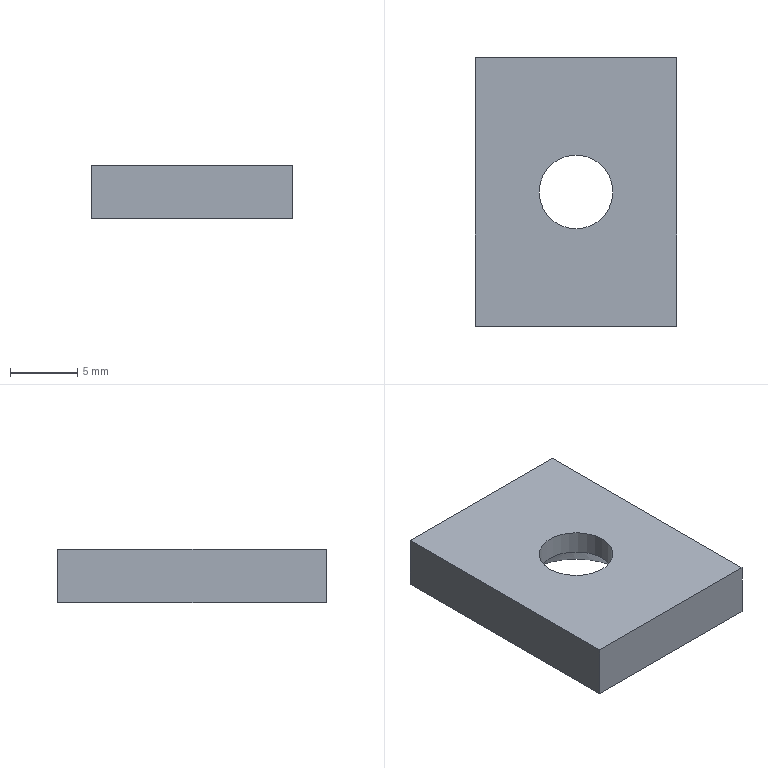Part | NX | features DATUM_CSYS 2, CSUNK_HOLE 1, EXTRUDE 1, HOLE PACKAGE 1, SKETCH 1 | 1 solid | 8 faces | box 15 x 20 x 4 mm | volume 1049 mm3 | plane 6 | cylinder 1 | cone 1 | commonest cylinder face diameters 5.5 x1
STEP:
#1=CARTESIAN_POINT('',(-7.5,10.,0.));
#2=VERTEX_POINT('',#1);
#3=CARTESIAN_POINT('',(-7.5,-10.,0.));
#4=VERTEX_POINT('',#3);
#5=CARTESIAN_POINT('',(-7.5,10.,0.));
#6=DIRECTION('',(0.,-1.,0.));
#7=VECTOR('',#6,1000.);
#8=LINE('',#5,#7);
#9=EDGE_CURVE('',#2,#4,#8,.T.);
#10=ORIENTED_EDGE('',*,*,#9,.T.);
#11=CARTESIAN_POINT('',(-7.5,-10.,4.));
#12=VERTEX_POINT('',#11);
#13=CARTESIAN_POINT('',(-7.5,-10.,4.));
#14=DIRECTION('',(0.,0.,-1.));
#15=VECTOR('',#14,1000.);
#16=LINE('',#13,#15);
#17=EDGE_CURVE('',#12,#4,#16,.T.);
#18=ORIENTED_EDGE('',*,*,#17,.F.);
#19=CARTESIAN_POINT('',(-7.5,10.,4.));
#20=VERTEX_POINT('',#19);
#21=CARTESIAN_POINT('',(-7.5,10.,4.));
#22=DIRECTION('',(0.,-1.,0.));
#23=VECTOR('',#22,1000.);
#24=LINE('',#21,#23);
#25=EDGE_CURVE('',#20,#12,#24,.T.);
#26=ORIENTED_EDGE('',*,*,#25,.F.);
#27=CARTESIAN_POINT('',(-7.5,10.,4.));
#28=DIRECTION('',(0.,0.,-1.));
#29=VECTOR('',#28,1000.);
#30=LINE('',#27,#29);
#31=EDGE_CURVE('',#20,#2,#30,.T.);
#32=ORIENTED_EDGE('',*,*,#31,.T.);
#33=EDGE_LOOP('',(#10,#18,#26,#32));
#34=FACE_BOUND('',#33,.T.);
#35=CARTESIAN_POINT('',(-7.5,10.,4.));
#36=DIRECTION('',(1.,0.,0.));
#37=DIRECTION('',(0.,1.,0.));
#38=AXIS2_PLACEMENT_3D('',#35,#36,#37);
#39=PLANE('',#38);
#40=ADVANCED_FACE('',(#34),#39,.F.);
#41=CARTESIAN_POINT('',(7.5,-10.,0.));
#42=VERTEX_POINT('',#41);
#43=CARTESIAN_POINT('',(-7.5,-10.,0.));
#44=DIRECTION('',(1.,0.,0.));
#45=VECTOR('',#44,1000.);
#46=LINE('',#43,#45);
#47=EDGE_CURVE('',#4,#42,#46,.T.);
#48=ORIENTED_EDGE('',*,*,#47,.T.);
#49=CARTESIAN_POINT('',(7.5,-10.,4.));
#50=VERTEX_POINT('',#49);
#51=CARTESIAN_POINT('',(7.5,-10.,4.));
#52=DIRECTION('',(0.,0.,-1.));
#53=VECTOR('',#52,1000.);
#54=LINE('',#51,#53);
#55=EDGE_CURVE('',#50,#42,#54,.T.);
#56=ORIENTED_EDGE('',*,*,#55,.F.);
#57=CARTESIAN_POINT('',(-7.5,-10.,4.));
#58=DIRECTION('',(1.,0.,0.));
#59=VECTOR('',#58,1000.);
#60=LINE('',#57,#59);
#61=EDGE_CURVE('',#12,#50,#60,.T.);
#62=ORIENTED_EDGE('',*,*,#61,.F.);
#63=ORIENTED_EDGE('',*,*,#17,.T.);
#64=EDGE_LOOP('',(#48,#56,#62,#63));
#65=FACE_BOUND('',#64,.T.);
#66=CARTESIAN_POINT('',(-7.5,-10.,4.));
#67=DIRECTION('',(0.,1.,0.));
#68=DIRECTION('',(-1.,0.,0.));
#69=AXIS2_PLACEMENT_3D('',#66,#67,#68);
#70=PLANE('',#69);
#71=ADVANCED_FACE('',(#65),#70,.F.);
#72=CARTESIAN_POINT('',(7.5,10.,0.));
#73=VERTEX_POINT('',#72);
#74=CARTESIAN_POINT('',(7.5,-10.,0.));
#75=DIRECTION('',(0.,1.,0.));
#76=VECTOR('',#75,1000.);
#77=LINE('',#74,#76);
#78=EDGE_CURVE('',#42,#73,#77,.T.);
#79=ORIENTED_EDGE('',*,*,#78,.T.);
#80=CARTESIAN_POINT('',(7.5,10.,4.));
#81=VERTEX_POINT('',#80);
#82=CARTESIAN_POINT('',(7.5,10.,4.));
#83=DIRECTION('',(0.,0.,-1.));
#84=VECTOR('',#83,1000.);
#85=LINE('',#82,#84);
#86=EDGE_CURVE('',#81,#73,#85,.T.);
#87=ORIENTED_EDGE('',*,*,#86,.F.);
#88=CARTESIAN_POINT('',(7.5,-10.,4.));
#89=DIRECTION('',(0.,1.,0.));
#90=VECTOR('',#89,1000.);
#91=LINE('',#88,#90);
#92=EDGE_CURVE('',#50,#81,#91,.T.);
#93=ORIENTED_EDGE('',*,*,#92,.F.);
#94=ORIENTED_EDGE('',*,*,#55,.T.);
#95=EDGE_LOOP('',(#79,#87,#93,#94));
#96=FACE_BOUND('',#95,.T.);
#97=CARTESIAN_POINT('',(7.5,-10.,4.));
#98=DIRECTION('',(-1.,0.,0.));
#99=DIRECTION('',(0.,-1.,0.));
#100=AXIS2_PLACEMENT_3D('',#97,#98,#99);
#101=PLANE('',#100);
#102=ADVANCED_FACE('',(#96),#101,.F.);
#103=CARTESIAN_POINT('',(7.5,10.,0.));
#104=DIRECTION('',(-1.,0.,0.));
#105=VECTOR('',#104,1000.);
#106=LINE('',#103,#105);
#107=EDGE_CURVE('',#73,#2,#106,.T.);
#108=ORIENTED_EDGE('',*,*,#107,.T.);
#109=ORIENTED_EDGE('',*,*,#31,.F.);
#110=CARTESIAN_POINT('',(7.5,10.,4.));
#111=DIRECTION('',(-1.,0.,0.));
#112=VECTOR('',#111,1000.);
#113=LINE('',#110,#112);
#114=EDGE_CURVE('',#81,#20,#113,.T.);
#115=ORIENTED_EDGE('',*,*,#114,.F.);
#116=ORIENTED_EDGE('',*,*,#86,.T.);
#117=EDGE_LOOP('',(#108,#109,#115,#116));
#118=FACE_BOUND('',#117,.T.);
#119=CARTESIAN_POINT('',(7.5,10.,4.));
#120=DIRECTION('',(0.,-1.,0.));
#121=DIRECTION('',(1.,0.,0.));
#122=AXIS2_PLACEMENT_3D('',#119,#120,#121);
#123=PLANE('',#122);
#124=ADVANCED_FACE('',(#118),#123,.F.);
#125=CARTESIAN_POINT('',(2.75,0.,4.));
#126=VERTEX_POINT('',#125);
#127=CARTESIAN_POINT('',(0.,0.,4.));
#128=DIRECTION('',(0.,0.,1.));
#129=DIRECTION('',(1.,0.,0.));
#130=AXIS2_PLACEMENT_3D('',#127,#128,#129);
#131=CIRCLE('',#130,2.75);
#132=EDGE_CURVE('',#126,#126,#131,.T.);
#133=ORIENTED_EDGE('',*,*,#132,.F.);
#134=EDGE_LOOP('',(#133));
#135=FACE_BOUND('',#134,.T.);
#136=ORIENTED_EDGE('',*,*,#25,.T.);
#137=ORIENTED_EDGE('',*,*,#61,.T.);
#138=ORIENTED_EDGE('',*,*,#92,.T.);
#139=ORIENTED_EDGE('',*,*,#114,.T.);
#140=EDGE_LOOP('',(#136,#137,#138,#139));
#141=FACE_BOUND('',#140,.T.);
#142=CARTESIAN_POINT('',(0.,0.,4.));
#143=DIRECTION('',(0.,0.,1.));
#144=DIRECTION('',(1.,0.,0.));
#145=AXIS2_PLACEMENT_3D('',#142,#143,#144);
#146=PLANE('',#145);
#147=ADVANCED_FACE('',(#135,#141),#146,.T.);
#148=CARTESIAN_POINT('',(5.,0.,0.));
#149=VERTEX_POINT('',#148);
#150=CARTESIAN_POINT('',(0.,0.,0.));
#151=DIRECTION('',(0.,0.,1.));
#152=DIRECTION('',(1.,0.,0.));
#153=AXIS2_PLACEMENT_3D('',#150,#151,#152);
#154=CIRCLE('',#153,5.);
#155=EDGE_CURVE('',#149,#149,#154,.T.);
#156=ORIENTED_EDGE('',*,*,#155,.T.);
#157=EDGE_LOOP('',(#156));
#158=FACE_BOUND('',#157,.T.);
#159=ORIENTED_EDGE('',*,*,#9,.F.);
#160=ORIENTED_EDGE('',*,*,#107,.F.);
#161=ORIENTED_EDGE('',*,*,#78,.F.);
#162=ORIENTED_EDGE('',*,*,#47,.F.);
#163=EDGE_LOOP('',(#159,#160,#161,#162));
#164=FACE_BOUND('',#163,.T.);
#165=CARTESIAN_POINT('',(0.,0.,0.));
#166=DIRECTION('',(0.,0.,1.));
#167=DIRECTION('',(1.,0.,0.));
#168=AXIS2_PLACEMENT_3D('',#165,#166,#167);
#169=PLANE('',#168);
#170=ADVANCED_FACE('',(#158,#164),#169,.F.);
#171=ORIENTED_EDGE('',*,*,#132,.T.);
#172=EDGE_LOOP('',(#171));
#173=FACE_BOUND('',#172,.T.);
#174=CARTESIAN_POINT('',(2.75,0.,2.25));
#175=VERTEX_POINT('',#174);
#176=CARTESIAN_POINT('',(0.,0.,2.25));
#177=DIRECTION('',(0.,0.,1.));
#178=DIRECTION('',(1.,0.,0.));
#179=AXIS2_PLACEMENT_3D('',#176,#177,#178);
#180=CIRCLE('',#179,2.75);
#181=EDGE_CURVE('',#175,#175,#180,.F.);
#182=ORIENTED_EDGE('',*,*,#181,.T.);
#183=EDGE_LOOP('',(#182));
#184=FACE_BOUND('',#183,.T.);
#185=CARTESIAN_POINT('',(0.,0.,15.925));
#186=DIRECTION('',(0.,0.,1.));
#187=DIRECTION('',(1.,0.,0.));
#188=AXIS2_PLACEMENT_3D('',#185,#186,#187);
#189=CYLINDRICAL_SURFACE('',#188,2.75);
#190=ADVANCED_FACE('',(#173,#184),#189,.F.);
#191=ORIENTED_EDGE('',*,*,#181,.F.);
#192=EDGE_LOOP('',(#191));
#193=FACE_BOUND('',#192,.T.);
#194=ORIENTED_EDGE('',*,*,#155,.F.);
#195=EDGE_LOOP('',(#194));
#196=FACE_BOUND('',#195,.T.);
#197=CARTESIAN_POINT('',(0.,0.,0.));
#198=DIRECTION('',(0.,0.,-1.));
#199=DIRECTION('',(-1.,0.,0.));
#200=AXIS2_PLACEMENT_3D('',#197,#198,#199);
#201=CONICAL_SURFACE('',#200,5.,0.7854);
#202=ADVANCED_FACE('',(#193,#196),#201,.F.);
#203=CLOSED_SHELL('',(#40,#71,#102,#124,#147,#170,#190,#202));
#204=MANIFOLD_SOLID_BREP('',#203);
#205=(LENGTH_UNIT()NAMED_UNIT(*)SI_UNIT(.MILLI.,.METRE.));
#206=UNCERTAINTY_MEASURE_WITH_UNIT(LENGTH_MEASURE(0.00001),#205,'','');
#207=(NAMED_UNIT(*)PLANE_ANGLE_UNIT()SI_UNIT($,.RADIAN.));
#208=(NAMED_UNIT(*)SI_UNIT($,.STERADIAN.)SOLID_ANGLE_UNIT());
#209=(GEOMETRIC_REPRESENTATION_CONTEXT(3)GLOBAL_UNCERTAINTY_ASSIGNED_CONTEXT((#206))GLOBAL_UNIT_ASSIGNED_CONTEXT((#205,#207,#208))REPRESENTATION_CONTEXT('',''));
#210=ADVANCED_BREP_SHAPE_REPRESENTATION('',(#204),#209);